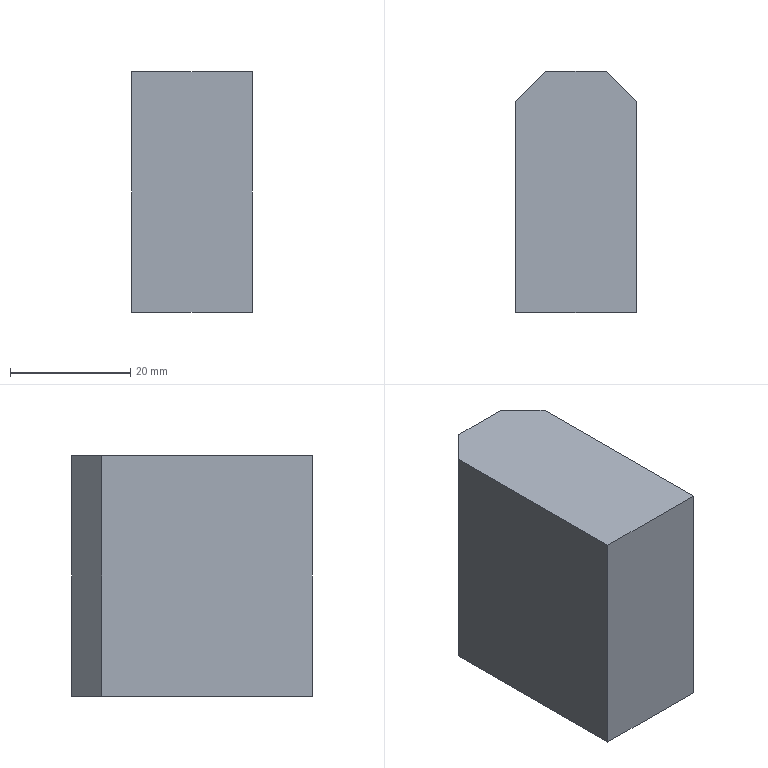Part | SolidWorks | features Chamfer 1, Extrusion 1 | 1 solid | 8 faces | box 20 x 40 x 40 mm | volume 31000 mm3 | plane 8
STEP:
#1=CARTESIAN_POINT('',(-10.,15.,40.));
#2=VERTEX_POINT('',#1);
#3=CARTESIAN_POINT('',(-10.,-20.,40.));
#4=VERTEX_POINT('',#3);
#5=CARTESIAN_POINT('',(-10.,20.,40.));
#6=DIRECTION('',(0.,-1.,0.));
#7=VECTOR('',#6,1000.);
#8=LINE('',#5,#7);
#9=EDGE_CURVE('',#2,#4,#8,.T.);
#10=ORIENTED_EDGE('',*,*,#9,.F.);
#11=CARTESIAN_POINT('',(-10.,15.,0.));
#12=VERTEX_POINT('',#11);
#13=CARTESIAN_POINT('',(-10.,15.,40.));
#14=DIRECTION('',(0.,0.,-1.));
#15=VECTOR('',#14,1000.);
#16=LINE('',#13,#15);
#17=EDGE_CURVE('',#2,#12,#16,.T.);
#18=ORIENTED_EDGE('',*,*,#17,.T.);
#19=CARTESIAN_POINT('',(-10.,-20.,0.));
#20=VERTEX_POINT('',#19);
#21=CARTESIAN_POINT('',(-10.,20.,0.));
#22=DIRECTION('',(0.,-1.,0.));
#23=VECTOR('',#22,1000.);
#24=LINE('',#21,#23);
#25=EDGE_CURVE('',#12,#20,#24,.T.);
#26=ORIENTED_EDGE('',*,*,#25,.T.);
#27=CARTESIAN_POINT('',(-10.,-20.,40.));
#28=DIRECTION('',(0.,0.,-1.));
#29=VECTOR('',#28,1000.);
#30=LINE('',#27,#29);
#31=EDGE_CURVE('',#4,#20,#30,.T.);
#32=ORIENTED_EDGE('',*,*,#31,.F.);
#33=EDGE_LOOP('',(#10,#18,#26,#32));
#34=FACE_OUTER_BOUND('',#33,.T.);
#35=CARTESIAN_POINT('',(-10.,20.,40.));
#36=DIRECTION('',(1.,0.,0.));
#37=DIRECTION('',(0.,1.,0.));
#38=AXIS2_PLACEMENT_3D('',#35,#36,#37);
#39=PLANE('',#38);
#40=ADVANCED_FACE('',(#34),#39,.F.);
#41=CARTESIAN_POINT('',(10.,-20.,0.));
#42=VERTEX_POINT('',#41);
#43=CARTESIAN_POINT('',(10.,-20.,0.));
#44=DIRECTION('',(1.,0.,0.));
#45=VECTOR('',#44,1000.);
#46=LINE('',#43,#45);
#47=EDGE_CURVE('',#20,#42,#46,.T.);
#48=ORIENTED_EDGE('',*,*,#47,.T.);
#49=CARTESIAN_POINT('',(10.,-20.,40.));
#50=VERTEX_POINT('',#49);
#51=CARTESIAN_POINT('',(10.,-20.,40.));
#52=DIRECTION('',(0.,0.,-1.));
#53=VECTOR('',#52,1000.);
#54=LINE('',#51,#53);
#55=EDGE_CURVE('',#50,#42,#54,.T.);
#56=ORIENTED_EDGE('',*,*,#55,.F.);
#57=CARTESIAN_POINT('',(10.,-20.,40.));
#58=DIRECTION('',(1.,0.,0.));
#59=VECTOR('',#58,1000.);
#60=LINE('',#57,#59);
#61=EDGE_CURVE('',#4,#50,#60,.T.);
#62=ORIENTED_EDGE('',*,*,#61,.F.);
#63=ORIENTED_EDGE('',*,*,#31,.T.);
#64=EDGE_LOOP('',(#48,#56,#62,#63));
#65=FACE_OUTER_BOUND('',#64,.T.);
#66=CARTESIAN_POINT('',(10.,-20.,40.));
#67=DIRECTION('',(0.,1.,0.));
#68=DIRECTION('',(0.,0.,1.));
#69=AXIS2_PLACEMENT_3D('',#66,#67,#68);
#70=PLANE('',#69);
#71=ADVANCED_FACE('',(#65),#70,.F.);
#72=CARTESIAN_POINT('',(10.,15.,0.));
#73=VERTEX_POINT('',#72);
#74=CARTESIAN_POINT('',(10.,20.,0.));
#75=DIRECTION('',(0.,1.,0.));
#76=VECTOR('',#75,1000.);
#77=LINE('',#74,#76);
#78=EDGE_CURVE('',#42,#73,#77,.T.);
#79=ORIENTED_EDGE('',*,*,#78,.T.);
#80=CARTESIAN_POINT('',(10.,15.,40.));
#81=VERTEX_POINT('',#80);
#82=CARTESIAN_POINT('',(10.,15.,40.));
#83=DIRECTION('',(0.,0.,1.));
#84=VECTOR('',#83,1000.);
#85=LINE('',#82,#84);
#86=EDGE_CURVE('',#73,#81,#85,.T.);
#87=ORIENTED_EDGE('',*,*,#86,.T.);
#88=CARTESIAN_POINT('',(10.,20.,40.));
#89=DIRECTION('',(0.,1.,0.));
#90=VECTOR('',#89,1000.);
#91=LINE('',#88,#90);
#92=EDGE_CURVE('',#50,#81,#91,.T.);
#93=ORIENTED_EDGE('',*,*,#92,.F.);
#94=ORIENTED_EDGE('',*,*,#55,.T.);
#95=EDGE_LOOP('',(#79,#87,#93,#94));
#96=FACE_OUTER_BOUND('',#95,.T.);
#97=CARTESIAN_POINT('',(10.,20.,40.));
#98=DIRECTION('',(-1.,0.,0.));
#99=DIRECTION('',(0.,-1.,0.));
#100=AXIS2_PLACEMENT_3D('',#97,#98,#99);
#101=PLANE('',#100);
#102=ADVANCED_FACE('',(#96),#101,.F.);
#103=CARTESIAN_POINT('',(5.,20.,0.));
#104=VERTEX_POINT('',#103);
#105=CARTESIAN_POINT('',(-5.,20.,0.));
#106=VERTEX_POINT('',#105);
#107=CARTESIAN_POINT('',(10.,20.,0.));
#108=DIRECTION('',(-1.,0.,0.));
#109=VECTOR('',#108,1000.);
#110=LINE('',#107,#109);
#111=EDGE_CURVE('',#104,#106,#110,.T.);
#112=ORIENTED_EDGE('',*,*,#111,.T.);
#113=CARTESIAN_POINT('',(-5.,20.,40.));
#114=VERTEX_POINT('',#113);
#115=CARTESIAN_POINT('',(-5.,20.,40.));
#116=DIRECTION('',(0.,0.,1.));
#117=VECTOR('',#116,1000.);
#118=LINE('',#115,#117);
#119=EDGE_CURVE('',#106,#114,#118,.T.);
#120=ORIENTED_EDGE('',*,*,#119,.T.);
#121=CARTESIAN_POINT('',(5.,20.,40.));
#122=VERTEX_POINT('',#121);
#123=CARTESIAN_POINT('',(10.,20.,40.));
#124=DIRECTION('',(-1.,0.,0.));
#125=VECTOR('',#124,1000.);
#126=LINE('',#123,#125);
#127=EDGE_CURVE('',#122,#114,#126,.T.);
#128=ORIENTED_EDGE('',*,*,#127,.F.);
#129=CARTESIAN_POINT('',(5.,20.,40.));
#130=DIRECTION('',(0.,0.,-1.));
#131=VECTOR('',#130,1000.);
#132=LINE('',#129,#131);
#133=EDGE_CURVE('',#122,#104,#132,.T.);
#134=ORIENTED_EDGE('',*,*,#133,.T.);
#135=EDGE_LOOP('',(#112,#120,#128,#134));
#136=FACE_OUTER_BOUND('',#135,.T.);
#137=CARTESIAN_POINT('',(10.,20.,40.));
#138=DIRECTION('',(0.,-1.,0.));
#139=DIRECTION('',(0.,0.,-1.));
#140=AXIS2_PLACEMENT_3D('',#137,#138,#139);
#141=PLANE('',#140);
#142=ADVANCED_FACE('',(#136),#141,.F.);
#143=ORIENTED_EDGE('',*,*,#127,.T.);
#144=CARTESIAN_POINT('',(-10.,15.,40.));
#145=DIRECTION('',(-0.7071,-0.7071,0.));
#146=VECTOR('',#145,1000.);
#147=LINE('',#144,#146);
#148=EDGE_CURVE('',#114,#2,#147,.T.);
#149=ORIENTED_EDGE('',*,*,#148,.T.);
#150=ORIENTED_EDGE('',*,*,#9,.T.);
#151=ORIENTED_EDGE('',*,*,#61,.T.);
#152=ORIENTED_EDGE('',*,*,#92,.T.);
#153=CARTESIAN_POINT('',(5.,20.,40.));
#154=DIRECTION('',(-0.7071,0.7071,0.));
#155=VECTOR('',#154,1000.);
#156=LINE('',#153,#155);
#157=EDGE_CURVE('',#81,#122,#156,.T.);
#158=ORIENTED_EDGE('',*,*,#157,.T.);
#159=EDGE_LOOP('',(#143,#149,#150,#151,#152,#158));
#160=FACE_OUTER_BOUND('',#159,.T.);
#161=CARTESIAN_POINT('',(0.,0.,40.));
#162=DIRECTION('',(0.,0.,-1.));
#163=DIRECTION('',(-1.,0.,0.));
#164=AXIS2_PLACEMENT_3D('',#161,#162,#163);
#165=PLANE('',#164);
#166=ADVANCED_FACE('',(#160),#165,.F.);
#167=ORIENTED_EDGE('',*,*,#25,.F.);
#168=CARTESIAN_POINT('',(-12.5,12.5,0.));
#169=DIRECTION('',(0.7071,0.7071,0.));
#170=VECTOR('',#169,1000.);
#171=LINE('',#168,#170);
#172=EDGE_CURVE('',#12,#106,#171,.T.);
#173=ORIENTED_EDGE('',*,*,#172,.T.);
#174=ORIENTED_EDGE('',*,*,#111,.F.);
#175=CARTESIAN_POINT('',(12.5,12.5,0.));
#176=DIRECTION('',(0.7071,-0.7071,0.));
#177=VECTOR('',#176,1000.);
#178=LINE('',#175,#177);
#179=EDGE_CURVE('',#104,#73,#178,.T.);
#180=ORIENTED_EDGE('',*,*,#179,.T.);
#181=ORIENTED_EDGE('',*,*,#78,.F.);
#182=ORIENTED_EDGE('',*,*,#47,.F.);
#183=EDGE_LOOP('',(#167,#173,#174,#180,#181,#182));
#184=FACE_OUTER_BOUND('',#183,.T.);
#185=CARTESIAN_POINT('',(0.,0.,0.));
#186=DIRECTION('',(0.,0.,-1.));
#187=DIRECTION('',(-1.,0.,0.));
#188=AXIS2_PLACEMENT_3D('',#185,#186,#187);
#189=PLANE('',#188);
#190=ADVANCED_FACE('',(#184),#189,.T.);
#191=ORIENTED_EDGE('',*,*,#148,.F.);
#192=ORIENTED_EDGE('',*,*,#119,.F.);
#193=ORIENTED_EDGE('',*,*,#172,.F.);
#194=ORIENTED_EDGE('',*,*,#17,.F.);
#195=EDGE_LOOP('',(#191,#192,#193,#194));
#196=FACE_OUTER_BOUND('',#195,.T.);
#197=CARTESIAN_POINT('',(-10.,15.,40.));
#198=DIRECTION('',(0.7071,-0.7071,0.));
#199=DIRECTION('',(0.,0.,-1.));
#200=AXIS2_PLACEMENT_3D('',#197,#198,#199);
#201=PLANE('',#200);
#202=ADVANCED_FACE('',(#196),#201,.F.);
#203=ORIENTED_EDGE('',*,*,#157,.F.);
#204=ORIENTED_EDGE('',*,*,#86,.F.);
#205=ORIENTED_EDGE('',*,*,#179,.F.);
#206=ORIENTED_EDGE('',*,*,#133,.F.);
#207=EDGE_LOOP('',(#203,#204,#205,#206));
#208=FACE_OUTER_BOUND('',#207,.T.);
#209=CARTESIAN_POINT('',(5.,20.,40.));
#210=DIRECTION('',(-0.7071,-0.7071,0.));
#211=DIRECTION('',(0.,0.,-1.));
#212=AXIS2_PLACEMENT_3D('',#209,#210,#211);
#213=PLANE('',#212);
#214=ADVANCED_FACE('',(#208),#213,.F.);
#215=CLOSED_SHELL('',(#40,#71,#102,#142,#166,#190,#202,#214));
#216=MANIFOLD_SOLID_BREP('',#215);
#217=CARTESIAN_POINT('',(0.,0.,0.));
#218=DIRECTION('',(0.,0.,1.));
#219=DIRECTION('',(1.,0.,0.));
#220=AXIS2_PLACEMENT_3D('',#217,#218,#219);
#221=(LENGTH_UNIT()NAMED_UNIT(*)SI_UNIT(.MILLI.,.METRE.));
#222=UNCERTAINTY_MEASURE_WITH_UNIT(LENGTH_MEASURE(0.00001),#221,'','');
#223=(NAMED_UNIT(*)PLANE_ANGLE_UNIT()SI_UNIT($,.RADIAN.));
#224=(NAMED_UNIT(*)SI_UNIT($,.STERADIAN.)SOLID_ANGLE_UNIT());
#225=(GEOMETRIC_REPRESENTATION_CONTEXT(3)GLOBAL_UNCERTAINTY_ASSIGNED_CONTEXT((#222))GLOBAL_UNIT_ASSIGNED_CONTEXT((#221,#223,#224))REPRESENTATION_CONTEXT('',''));
#226=ADVANCED_BREP_SHAPE_REPRESENTATION('',(#216,#220),#225);